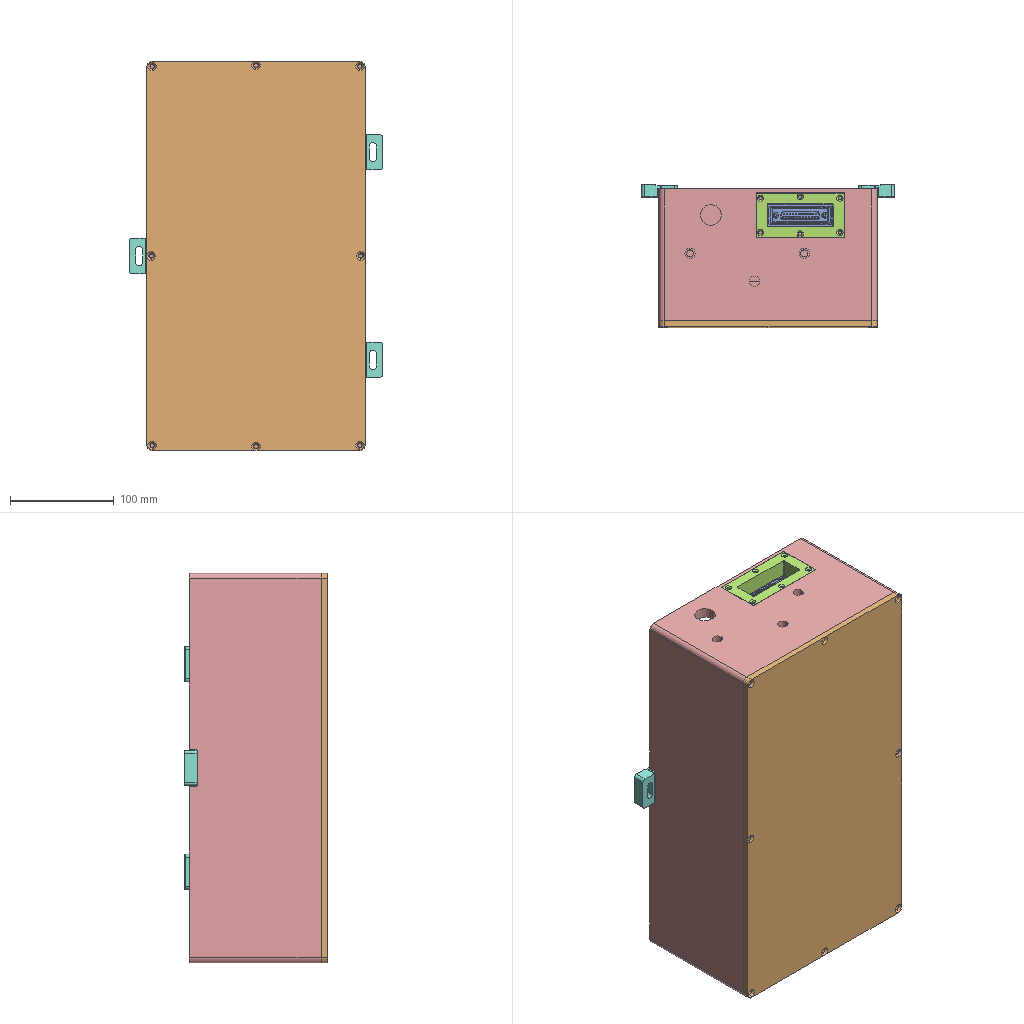Assembly | SolidWorks | 6 different items | 8 placed | box 244 x 138 x 375 mm
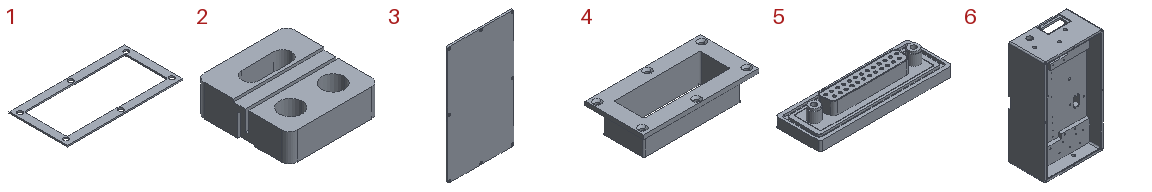Parts list (item | quantity | size | volume | features):
1 | x1 | 83.5 x 42 x 1 mm | 1203 mm3 | features Extrusion 1, Fillet 1
2 | x3 | 34 x 35 x 12 mm | 10318 mm3 | features ICE 7, Extrusion 1, Fillet 1
3 | x1 | 210 x 6 x 375 mm | 471315 mm3 | features ICE 42, Fillet 8, DeleteBody 2, Cut 1, Extrusion 1, HoleWzd 1, MoveFace 1, RefAxis 1
4 | x1 | 84.5 x 43 x 21 mm | 19535 mm3 | features ICE 3, Fillet 2, Extrusion 1, HoleWzd 1
5 | x1 | 62.5 x 21 x 10.6 mm | 7477 mm3 | features BaseBody 1
6 | x1 | 210 x 127 x 375 mm | 3262680 mm3 | features ICE 39, Fillet 6, MoveFace 4, Cut 3, Extrusion 1
Mates (type | each side: item.copy, entity, surface, feature):
Coincident | 4.1 face plane Boss-Extrude2 | 1.1 face plane Boss-Extrude1
Concentric | 4.1 face cylinder Cut-Extrude2 | 1.1 face cylinder Boss-Extrude1 | 2 times
Coincident | 6.1 face plane Boss-Extrude3 | 3.1 face plane Boss-Extrude9
Concentric | 6.1 face cylinder Cut-Extrude22 | 3.1 face cylinder CSK for M4 Hex Socket Countersunk Cap Screw1 | 2 times
Concentric | 6.1 face cylinder Cut-Extrude32 | 2.1 face cylinder Cut-Extrude1 | 2 times
Coincident | 6.1 face plane Cut-Extrude31 | 2.1 face plane Cut-Extrude3
Concentric | 6.1 face cylinder Cut-Extrude32 | 2.2 face cylinder Cut-Extrude5
Concentric | 6.1 face cylinder Cut-Extrude32 | 2.2 face cylinder Cut-Extrude1
Coincident | 2.1 face plane Cut-Extrude2 | 2.2 face plane Cut-Extrude2
Coincident | 6.1 face plane Cut-Extrude31 | 2.3 face plane Cut-Extrude3
Concentric | 6.1 face cylinder Cut-Extrude32 | 2.3 face cylinder Cut-Extrude5
Concentric | 6.1 face cylinder Cut-Extrude32 | 2.3 face cylinder Cut-Extrude1